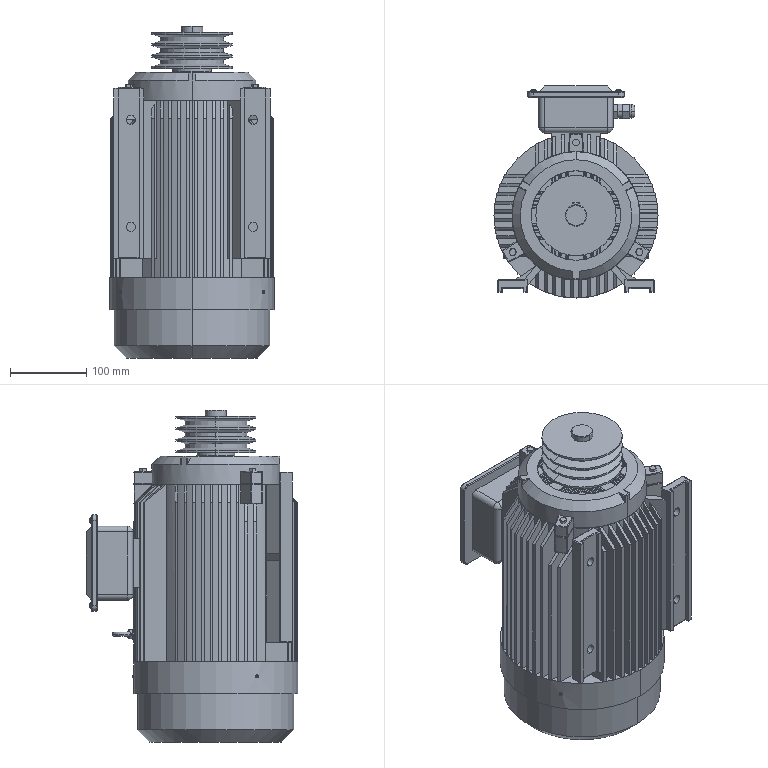Part | SolidWorks | 3 solids | 927 faces | box 215 x 277.5 x 435 mm | volume 11973483 mm3 | plane 459 | cylinder 274 | cone 89 | sphere 52 | torus 45 | spline 8 | commonest cylinder face diameters 2 x124 215 x48 14.555 x12 2.175 x8 7.277 x8 12 x8